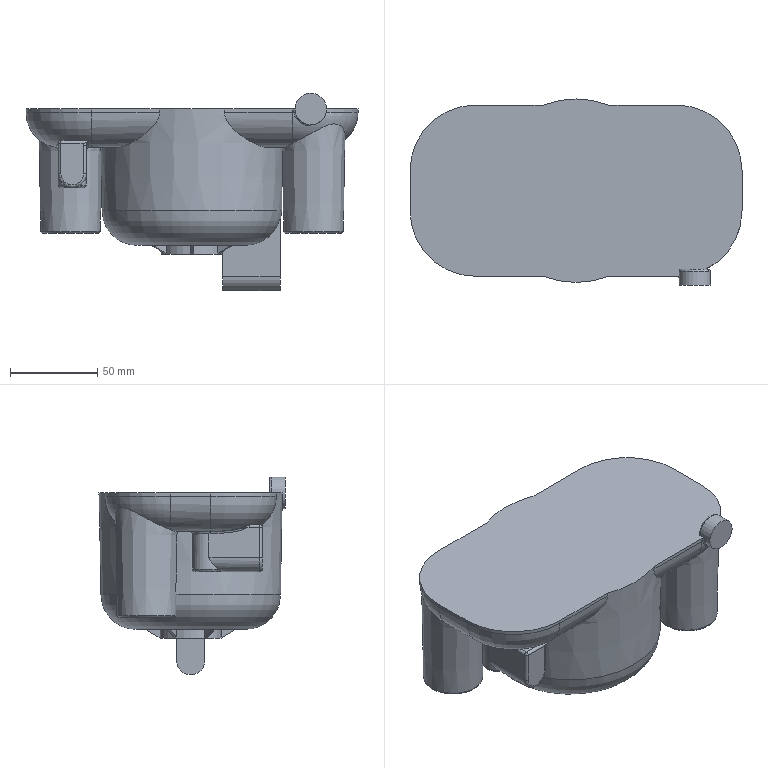Part | STEP file | Lower_shell_0 | 1 solid | 99 faces | box 190 x 106.5 x 113 mm | volume 927273 mm3 | plane 46 | cylinder 28 | spline 10 | torus 7 | other 4 | cone 3 | sphere 1 | commonest cylinder face diameters 3 x6 35 x6 40 x6 75 x5 16 x3 18 x1